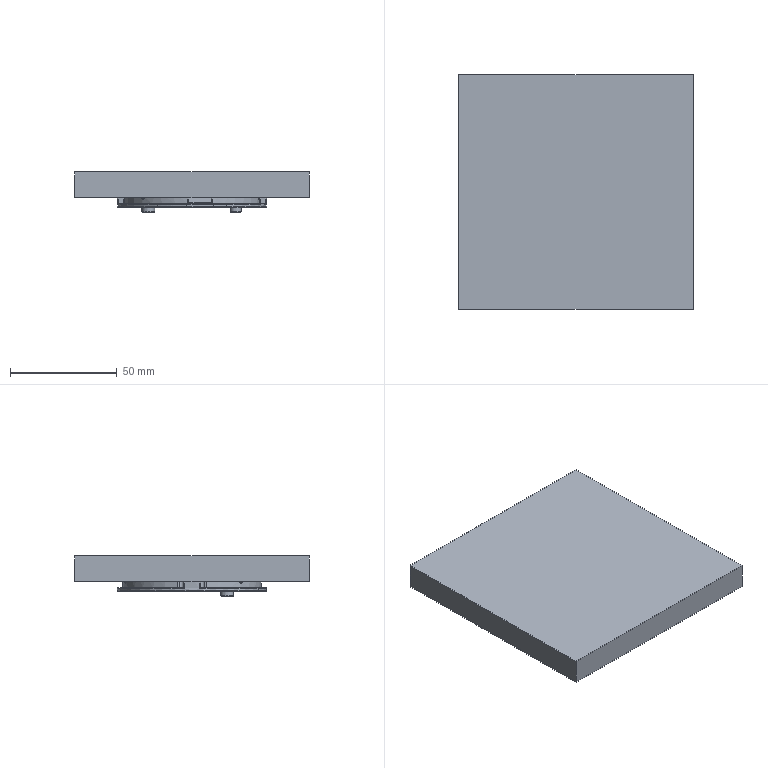NC program | NX | posted with a generic post | part box 110 x 110 x 18.8 mm
Lines 2503 to 3319 of 8004:
(ZLEVEL_PROFILE_1_COPY_1_COPY_COPY , TOOL : D2)
N4962 T02 M6
N4964 G54
N4966 G17 G0 G90 X-14.75 Y-12.131 S9500 M3
N4968 G43 Z30. H2
N4970 Z-2.8
N4972 G94 G1 Y-16.5 Z-3.029 F1000.
N4974 X-12.005 Z-3.173
N4976 X-12. Y-16.474 Z-3.174
N4978 Y-7.958 Z-3.621
N4980 X-12.053 Y-7.968 Z-3.623
N4982 X-12.32 Y-8.06 Z-3.638
N4984 X-12.965 Y-8.408 Z-3.677
N4986 X-13.537 Y-8.866 Z-3.715
N4988 X-14.015 Y-9.422 Z-3.753
N4990 X-14.384 Y-10.054 Z-3.792
N4992 X-14.632 Y-10.744 Z-3.83
N4994 X-14.75 Y-11.467 Z-3.869
N4996 Y-16.5 Z-4.132
N4998 X-12.005 Z-4.276
N5000 X-12. Y-16.474 Z-4.278
N5002 Y-12.229 Z-4.5
N5004 Y-7.958
N5006 X-12.053 Y-7.968
N5008 G3 X-14.75 Y-11.75 R4.
N5010 G1 Y-16.5
N5012 X-12.005
N5014 X-12. Y-16.474
N5016 Y-12.229
N5018 Y-8.081 Z-4.572
N5020 X-12.005 Y-7.962 Z-4.575
N5022 X-12.071 Y-7.981 Z-4.576
N5024 X-12.165 Y-8.011 Z-4.578
N5026 X-12.255 Y-8.051 Z-4.579
N5028 X-12.345 Y-8.092 Z-4.581
N5030 X-12.435 Y-8.132 Z-4.583
N5032 X-12.525 Y-8.172 Z-4.584
N5034 X-12.615 Y-8.213 Z-4.586
N5036 X-12.699 Y-8.265 Z-4.588
N5038 X-12.784 Y-8.316 Z-4.59
N5040 X-12.868 Y-8.367 Z-4.591
N5042 X-12.953 Y-8.418 Z-4.593
N5044 X-13.036 Y-8.471 Z-4.595
N5046 X-13.113 Y-8.532 Z-4.597
N5048 X-13.191 Y-8.593 Z-4.598
N5050 X-13.269 Y-8.653 Z-4.6
N5052 X-13.346 Y-8.714 Z-4.602
N5054 X-13.422 Y-8.778 Z-4.603
N5056 X-13.492 Y-8.848 Z-4.605
N5058 X-13.562 Y-8.917 Z-4.607
N5060 X-13.631 Y-8.987 Z-4.609
N5062 X-13.701 Y-9.057 Z-4.61
N5064 X-13.767 Y-9.13 Z-4.612
N5066 X-13.828 Y-9.207 Z-4.614
N5068 X-13.889 Y-9.285 Z-4.616
N5070 X-13.95 Y-9.363 Z-4.617
N5072 X-14.011 Y-9.44 Z-4.619
N5074 X-14.067 Y-9.521 Z-4.621
N5076 X-14.117 Y-9.606 Z-4.622
N5078 X-14.169 Y-9.69 Z-4.624
N5080 X-14.219 Y-9.775 Z-4.626
N5082 X-14.27 Y-9.859 Z-4.628
N5084 X-14.315 Y-9.947 Z-4.629
N5086 X-14.356 Y-10.037 Z-4.631
N5088 X-14.396 Y-10.127 Z-4.633
N5090 X-14.437 Y-10.217 Z-4.634
N5092 X-14.477 Y-10.307 Z-4.636
N5094 X-14.509 Y-10.4 Z-4.638
N5096 X-14.539 Y-10.494 Z-4.64
N5098 X-14.568 Y-10.588 Z-4.641
N5100 X-14.598 Y-10.683 Z-4.643
N5102 X-14.627 Y-10.777 Z-4.645
N5104 X-14.647 Y-10.873 Z-4.647
N5106 X-14.664 Y-10.971 Z-4.648
N5108 X-14.682 Y-11.068 Z-4.65
N5110 X-14.7 Y-11.164 Z-4.652
N5112 X-14.718 Y-11.262 Z-4.653
N5114 X-14.725 Y-11.36 Z-4.655
N5116 X-14.731 Y-11.459 Z-4.657
N5118 X-14.737 Y-11.557 Z-4.659
N5120 X-14.743 Y-11.656 Z-4.66
N5122 X-14.748 Y-11.754 Z-4.662
N5124 X-14.75 Y-11.853 Z-4.664
N5126 Y-13.927 Z-4.7
N5128 Y-16.483
N5130 X-14.745 Y-16.5
N5132 X-12.005
N5134 X-12. Y-16.474
N5136 Y-12.229
N5138 Y-8.081 Z-4.772
N5140 X-12.005 Y-7.962 Z-4.775
N5142 X-12.071 Y-7.981 Z-4.776
N5144 X-12.165 Y-8.011 Z-4.778
N5146 X-12.255 Y-8.051 Z-4.779
N5148 X-12.345 Y-8.092 Z-4.781
N5150 X-12.435 Y-8.132 Z-4.783
N5152 X-12.525 Y-8.172 Z-4.784
N5154 X-12.615 Y-8.213 Z-4.786
N5156 X-12.699 Y-8.265 Z-4.788
N5158 X-12.784 Y-8.316 Z-4.79
N5160 X-12.868 Y-8.367 Z-4.791
N5162 X-12.953 Y-8.418 Z-4.793
N5164 X-13.036 Y-8.471 Z-4.795
N5166 X-13.113 Y-8.532 Z-4.797
N5168 X-13.191 Y-8.593 Z-4.798
N5170 X-13.269 Y-8.653 Z-4.8
N5172 X-13.346 Y-8.714 Z-4.802
N5174 X-13.422 Y-8.778 Z-4.803
N5176 X-13.492 Y-8.848 Z-4.805
N5178 X-13.562 Y-8.917 Z-4.807
N5180 X-13.631 Y-8.987 Z-4.809
N5182 X-13.701 Y-9.057 Z-4.81
N5184 X-13.767 Y-9.13 Z-4.812
N5186 X-13.828 Y-9.207 Z-4.814
N5188 X-13.889 Y-9.285 Z-4.816
N5190 X-13.95 Y-9.363 Z-4.817
N5192 X-14.011 Y-9.44 Z-4.819
N5194 X-14.067 Y-9.521 Z-4.821
N5196 X-14.117 Y-9.606 Z-4.822
N5198 X-14.169 Y-9.69 Z-4.824
N5200 X-14.219 Y-9.775 Z-4.826
N5202 X-14.27 Y-9.859 Z-4.828
N5204 X-14.315 Y-9.947 Z-4.829
N5206 X-14.356 Y-10.037 Z-4.831
N5208 X-14.396 Y-10.127 Z-4.833
N5210 X-14.437 Y-10.217 Z-4.834
N5212 X-14.477 Y-10.307 Z-4.836
N5214 X-14.509 Y-10.4 Z-4.838
N5216 X-14.539 Y-10.494 Z-4.84
N5218 X-14.568 Y-10.588 Z-4.841
N5220 X-14.598 Y-10.683 Z-4.843
N5222 X-14.627 Y-10.777 Z-4.845
N5224 X-14.647 Y-10.873 Z-4.847
N5226 X-14.664 Y-10.971 Z-4.848
N5228 X-14.682 Y-11.068 Z-4.85
N5230 X-14.7 Y-11.164 Z-4.852
N5232 X-14.718 Y-11.262 Z-4.853
N5234 X-14.725 Y-11.36 Z-4.855
N5236 X-14.731 Y-11.459 Z-4.857
N5238 X-14.737 Y-11.557 Z-4.859
N5240 X-14.743 Y-11.656 Z-4.86
N5242 X-14.748 Y-11.754 Z-4.862
N5244 X-14.75 Y-11.853 Z-4.864
N5246 Y-13.927 Z-4.9
N5248 Y-16.483
N5250 X-14.745 Y-16.5
N5252 X-12.005
N5254 X-12. Y-16.474
N5256 Y-12.229
N5258 Y-8.081 Z-4.972
N5260 X-12.005 Y-7.962 Z-4.975
N5262 X-12.071 Y-7.981 Z-4.976
N5264 X-12.165 Y-8.011 Z-4.978
N5266 X-12.255 Y-8.051 Z-4.979
N5268 X-12.345 Y-8.092 Z-4.981
N5270 X-12.435 Y-8.132 Z-4.983
N5272 X-12.525 Y-8.172 Z-4.984
N5274 X-12.615 Y-8.213 Z-4.986
N5276 X-12.699 Y-8.265 Z-4.988
N5278 X-12.784 Y-8.316 Z-4.99
N5280 X-12.868 Y-8.367 Z-4.991
N5282 X-12.953 Y-8.418 Z-4.993
N5284 X-13.036 Y-8.471 Z-4.995
N5286 X-13.113 Y-8.532 Z-4.997
N5288 X-13.191 Y-8.593 Z-4.998
N5290 X-13.269 Y-8.653 Z-5.
N5292 X-13.346 Y-8.714 Z-5.002
N5294 X-13.422 Y-8.778 Z-5.003
N5296 X-13.492 Y-8.848 Z-5.005
N5298 X-13.562 Y-8.917 Z-5.007
N5300 X-13.631 Y-8.987 Z-5.009
N5302 X-13.701 Y-9.057 Z-5.01
N5304 X-13.767 Y-9.13 Z-5.012
N5306 X-13.828 Y-9.207 Z-5.014
N5308 X-13.889 Y-9.285 Z-5.016
N5310 X-13.95 Y-9.363 Z-5.017
N5312 X-14.011 Y-9.44 Z-5.019
N5314 X-14.067 Y-9.521 Z-5.021
N5316 X-14.117 Y-9.606 Z-5.022
N5318 X-14.169 Y-9.69 Z-5.024
N5320 X-14.219 Y-9.775 Z-5.026
N5322 X-14.27 Y-9.859 Z-5.028
N5324 X-14.315 Y-9.947 Z-5.029
N5326 X-14.356 Y-10.037 Z-5.031
N5328 X-14.396 Y-10.127 Z-5.033
N5330 X-14.437 Y-10.217 Z-5.034
N5332 X-14.477 Y-10.307 Z-5.036
N5334 X-14.509 Y-10.4 Z-5.038
N5336 X-14.539 Y-10.494 Z-5.04
N5338 X-14.568 Y-10.588 Z-5.041
N5340 X-14.598 Y-10.683 Z-5.043
N5342 X-14.627 Y-10.777 Z-5.045
N5344 X-14.647 Y-10.873 Z-5.047
N5346 X-14.664 Y-10.971 Z-5.048
N5348 X-14.682 Y-11.068 Z-5.05
N5350 X-14.7 Y-11.165 Z-5.052
N5352 X-14.718 Y-11.262 Z-5.053
N5354 X-14.724 Y-11.36 Z-5.055
N5356 X-14.731 Y-11.459 Z-5.057
N5358 X-14.737 Y-11.557 Z-5.059
N5360 X-14.743 Y-11.656 Z-5.06
N5362 X-14.748 Y-11.754 Z-5.062
N5364 X-14.75 Y-11.853 Z-5.064
N5366 Y-13.927 Z-5.1
N5368 Y-16.483
N5370 X-14.745 Y-16.5
N5372 X-12.005
N5374 X-12. Y-16.474
N5376 Y-12.229
N5378 Y-8.081 Z-5.172
N5380 X-12.005 Y-7.962 Z-5.175
N5382 X-12.071 Y-7.981 Z-5.176
N5384 X-12.165 Y-8.011 Z-5.178
N5386 X-12.255 Y-8.051 Z-5.179
N5388 X-12.345 Y-8.092 Z-5.181
N5390 X-12.435 Y-8.132 Z-5.183
N5392 X-12.525 Y-8.172 Z-5.184
N5394 X-12.615 Y-8.213 Z-5.186
N5396 X-12.699 Y-8.265 Z-5.188
N5398 X-12.784 Y-8.316 Z-5.19
N5400 X-12.868 Y-8.367 Z-5.191
N5402 X-12.953 Y-8.418 Z-5.193
N5404 X-13.036 Y-8.471 Z-5.195
N5406 X-13.113 Y-8.532 Z-5.197
N5408 X-13.191 Y-8.593 Z-5.198
N5410 X-13.269 Y-8.653 Z-5.2
N5412 X-13.346 Y-8.714 Z-5.202
N5414 X-13.422 Y-8.778 Z-5.203
N5416 X-13.491 Y-8.848 Z-5.205
N5418 X-13.562 Y-8.917 Z-5.207
N5420 X-13.631 Y-8.987 Z-5.209
N5422 X-13.701 Y-9.057 Z-5.21
N5424 X-13.767 Y-9.13 Z-5.212
N5426 X-13.828 Y-9.207 Z-5.214
N5428 X-13.889 Y-9.285 Z-5.216
N5430 X-13.95 Y-9.363 Z-5.217
N5432 X-14.011 Y-9.44 Z-5.219
N5434 X-14.067 Y-9.521 Z-5.221
N5436 X-14.117 Y-9.606 Z-5.222
N5438 X-14.169 Y-9.69 Z-5.224
N5440 X-14.219 Y-9.775 Z-5.226
N5442 X-14.27 Y-9.859 Z-5.228
N5444 X-14.315 Y-9.947 Z-5.229
N5446 X-14.356 Y-10.037 Z-5.231
N5448 X-14.396 Y-10.127 Z-5.233
N5450 X-14.437 Y-10.217 Z-5.234
N5452 X-14.477 Y-10.307 Z-5.236
N5454 X-14.509 Y-10.4 Z-5.238
N5456 X-14.539 Y-10.494 Z-5.24
N5458 X-14.568 Y-10.588 Z-5.241
N5460 X-14.598 Y-10.683 Z-5.243
N5462 X-14.627 Y-10.777 Z-5.245
N5464 X-14.647 Y-10.873 Z-5.247
N5466 X-14.664 Y-10.971 Z-5.248
N5468 X-14.682 Y-11.068 Z-5.25
N5470 X-14.7 Y-11.165 Z-5.252
N5472 X-14.718 Y-11.262 Z-5.253
N5474 X-14.724 Y-11.36 Z-5.255
N5476 X-14.731 Y-11.459 Z-5.257
N5478 X-14.737 Y-11.557 Z-5.259
N5480 X-14.743 Y-11.656 Z-5.26
N5482 X-14.748 Y-11.754 Z-5.262
N5484 X-14.75 Y-11.853 Z-5.264
N5486 Y-13.927 Z-5.3
N5488 Y-16.483
N5490 X-14.745 Y-16.5
N5492 X-12.005
N5494 X-12. Y-16.474
N5496 Y-12.229
N5498 Y-8.081 Z-5.372
N5500 X-12.005 Y-7.962 Z-5.375
N5502 X-12.071 Y-7.981 Z-5.376
N5504 X-12.165 Y-8.011 Z-5.378
N5506 X-12.255 Y-8.051 Z-5.379
N5508 X-12.346 Y-8.091 Z-5.381
N5510 X-12.435 Y-8.132 Z-5.383
N5512 X-12.525 Y-8.172 Z-5.384
N5514 X-12.615 Y-8.213 Z-5.386
N5516 X-12.699 Y-8.265 Z-5.388
N5518 X-12.784 Y-8.316 Z-5.39
N5520 X-12.868 Y-8.367 Z-5.391
N5522 X-12.953 Y-8.418 Z-5.393
N5524 X-13.036 Y-8.471 Z-5.395
N5526 X-13.113 Y-8.532 Z-5.397
N5528 X-13.191 Y-8.593 Z-5.398
N5530 X-13.269 Y-8.653 Z-5.4
N5532 X-13.346 Y-8.714 Z-5.402
N5534 X-13.422 Y-8.778 Z-5.403
N5536 X-13.491 Y-8.848 Z-5.405
N5538 X-13.562 Y-8.917 Z-5.407
N5540 X-13.631 Y-8.987 Z-5.409
N5542 X-13.701 Y-9.057 Z-5.41
N5544 X-13.767 Y-9.13 Z-5.412
N5546 X-13.828 Y-9.207 Z-5.414
N5548 X-13.889 Y-9.285 Z-5.416
N5550 X-13.95 Y-9.363 Z-5.417
N5552 X-14.011 Y-9.44 Z-5.419
N5554 X-14.067 Y-9.521 Z-5.421
N5556 X-14.117 Y-9.606 Z-5.422
N5558 X-14.169 Y-9.69 Z-5.424
N5560 X-14.219 Y-9.775 Z-5.426
N5562 X-14.27 Y-9.859 Z-5.428
N5564 X-14.315 Y-9.947 Z-5.429
N5566 X-14.356 Y-10.037 Z-5.431
N5568 X-14.396 Y-10.127 Z-5.433
N5570 X-14.437 Y-10.217 Z-5.434
N5572 X-14.477 Y-10.307 Z-5.436
N5574 X-14.509 Y-10.4 Z-5.438
N5576 X-14.539 Y-10.495 Z-5.44
N5578 X-14.568 Y-10.588 Z-5.441
N5580 X-14.597 Y-10.683 Z-5.443
N5582 X-14.627 Y-10.777 Z-5.445
N5584 X-14.647 Y-10.873 Z-5.447
N5586 X-14.664 Y-10.971 Z-5.448
N5588 X-14.682 Y-11.068 Z-5.45
N5590 X-14.7 Y-11.165 Z-5.452
N5592 X-14.718 Y-11.262 Z-5.453
N5594 X-14.724 Y-11.36 Z-5.455
N5596 X-14.731 Y-11.459 Z-5.457
N5598 X-14.737 Y-11.557 Z-5.459
N5600 X-14.743 Y-11.656 Z-5.46
N5602 X-14.748 Y-11.754 Z-5.462
N5604 X-14.75 Y-11.853 Z-5.464
N5606 Y-13.927 Z-5.5
N5608 Y-16.483
N5610 X-14.745 Y-16.5
N5612 X-12.005
N5614 X-12. Y-16.474
N5616 Y-12.229
N5618 Y-8.081 Z-5.572
N5620 X-12.005 Y-7.962 Z-5.575
N5622 X-12.071 Y-7.981 Z-5.576
N5624 X-12.165 Y-8.011 Z-5.578
N5626 X-12.255 Y-8.051 Z-5.579
N5628 X-12.346 Y-8.091 Z-5.581
N5630 X-12.435 Y-8.132 Z-5.583
N5632 X-12.525 Y-8.172 Z-5.584
N5634 X-12.615 Y-8.213 Z-5.586
N5636 X-12.699 Y-8.265 Z-5.588
N5638 X-12.784 Y-8.316 Z-5.59
N5640 X-12.868 Y-8.367 Z-5.591
N5642 X-12.953 Y-8.418 Z-5.593
N5644 X-13.036 Y-8.471 Z-5.595
N5646 X-13.113 Y-8.532 Z-5.597
N5648 X-13.191 Y-8.593 Z-5.598
N5650 X-13.269 Y-8.653 Z-5.6
N5652 X-13.346 Y-8.714 Z-5.602
N5654 X-13.422 Y-8.778 Z-5.603
N5656 X-13.491 Y-8.848 Z-5.605
N5658 X-13.562 Y-8.917 Z-5.607
N5660 X-13.631 Y-8.987 Z-5.609
N5662 X-13.701 Y-9.057 Z-5.61
N5664 X-13.767 Y-9.13 Z-5.612
N5666 X-13.828 Y-9.207 Z-5.614
N5668 X-13.889 Y-9.285 Z-5.616
N5670 X-13.95 Y-9.363 Z-5.617
N5672 X-14.011 Y-9.44 Z-5.619
N5674 X-14.067 Y-9.522 Z-5.621
N5676 X-14.117 Y-9.606 Z-5.622
N5678 X-14.169 Y-9.69 Z-5.624
N5680 X-14.219 Y-9.775 Z-5.626
N5682 X-14.27 Y-9.859 Z-5.628
N5684 X-14.315 Y-9.947 Z-5.629
N5686 X-14.356 Y-10.037 Z-5.631
N5688 X-14.396 Y-10.127 Z-5.633
N5690 X-14.437 Y-10.217 Z-5.634
N5692 X-14.477 Y-10.307 Z-5.636
N5694 X-14.509 Y-10.4 Z-5.638
N5696 X-14.539 Y-10.495 Z-5.64
N5698 X-14.568 Y-10.589 Z-5.641
N5700 X-14.597 Y-10.683 Z-5.643
N5702 X-14.627 Y-10.777 Z-5.645
N5704 X-14.647 Y-10.874 Z-5.647
N5706 X-14.664 Y-10.971 Z-5.648
N5708 X-14.682 Y-11.068 Z-5.65
N5710 X-14.7 Y-11.165 Z-5.652
N5712 X-14.718 Y-11.262 Z-5.653
N5714 X-14.724 Y-11.36 Z-5.655
N5716 X-14.731 Y-11.459 Z-5.657
N5718 X-14.737 Y-11.557 Z-5.659
N5720 X-14.743 Y-11.656 Z-5.66
N5722 X-14.748 Y-11.754 Z-5.662
N5724 X-14.75 Y-11.853 Z-5.664
N5726 Y-13.927 Z-5.7
N5728 Y-16.483
N5730 X-14.745 Y-16.5
N5732 X-12.005
N5734 X-12. Y-16.474
N5736 Y-12.229
N5738 Y-8.081 Z-5.772
N5740 X-12.005 Y-7.962 Z-5.775
N5742 X-12.071 Y-7.981 Z-5.776
N5744 X-12.165 Y-8.011 Z-5.778
N5746 X-12.255 Y-8.051 Z-5.779
N5748 X-12.346 Y-8.091 Z-5.781
N5750 X-12.435 Y-8.132 Z-5.783
N5752 X-12.525 Y-8.172 Z-5.784
N5754 X-12.615 Y-8.213 Z-5.786
N5756 X-12.699 Y-8.265 Z-5.788
N5758 X-12.784 Y-8.316 Z-5.79
N5760 X-12.868 Y-8.367 Z-5.791
N5762 X-12.953 Y-8.418 Z-5.793
N5764 X-13.036 Y-8.471 Z-5.795
N5766 X-13.113 Y-8.532 Z-5.797
N5768 X-13.191 Y-8.593 Z-5.798
N5770 X-13.269 Y-8.653 Z-5.8
N5772 X-13.346 Y-8.714 Z-5.802
N5774 X-13.422 Y-8.778 Z-5.803
N5776 X-13.491 Y-8.848 Z-5.805
N5778 X-13.562 Y-8.917 Z-5.807
N5780 X-13.631 Y-8.987 Z-5.809
N5782 X-13.701 Y-9.057 Z-5.81
N5784 X-13.767 Y-9.13 Z-5.812
N5786 X-13.828 Y-9.207 Z-5.814
N5788 X-13.889 Y-9.285 Z-5.816
N5790 X-13.95 Y-9.363 Z-5.817
N5792 X-14.011 Y-9.44 Z-5.819
N5794 X-14.067 Y-9.522 Z-5.821
N5796 X-14.117 Y-9.606 Z-5.822
N5798 X-14.169 Y-9.69 Z-5.824
N5800 X-14.219 Y-9.775 Z-5.826
N5802 X-14.27 Y-9.859 Z-5.828
N5804 X-14.315 Y-9.947 Z-5.829
N5806 X-14.356 Y-10.037 Z-5.831
N5808 X-14.396 Y-10.127 Z-5.833
N5810 X-14.437 Y-10.217 Z-5.834
N5812 X-14.477 Y-10.307 Z-5.836
N5814 X-14.509 Y-10.4 Z-5.838
N5816 X-14.539 Y-10.494 Z-5.84
N5818 X-14.568 Y-10.589 Z-5.841
N5820 X-14.597 Y-10.683 Z-5.843
N5822 X-14.627 Y-10.777 Z-5.845
N5824 X-14.647 Y-10.874 Z-5.847
N5826 X-14.664 Y-10.971 Z-5.848
N5828 X-14.682 Y-11.068 Z-5.85
N5830 X-14.7 Y-11.165 Z-5.852
N5832 X-14.718 Y-11.262 Z-5.853
N5834 X-14.724 Y-11.36 Z-5.855
N5836 X-14.731 Y-11.459 Z-5.857
N5838 X-14.736 Y-11.557 Z-5.859
N5840 X-14.743 Y-11.656 Z-5.86
N5842 X-14.748 Y-11.754 Z-5.862
N5844 X-14.75 Y-11.853 Z-5.864
N5846 Y-13.927 Z-5.9
N5848 Y-16.483
N5850 X-14.745 Y-16.5
N5852 X-12.005
N5854 X-12. Y-16.474
N5856 Y-12.229
N5858 Y-8.081 Z-5.972
N5860 X-12.005 Y-7.962 Z-5.975
N5862 X-12.071 Y-7.981 Z-5.976
N5864 X-12.165 Y-8.011 Z-5.978
N5866 X-12.255 Y-8.051 Z-5.979
N5868 X-12.346 Y-8.091 Z-5.981
N5870 X-12.435 Y-8.132 Z-5.983
N5872 X-12.525 Y-8.172 Z-5.984
N5874 X-12.615 Y-8.213 Z-5.986
N5876 X-12.699 Y-8.265 Z-5.988
N5878 X-12.784 Y-8.316 Z-5.99
N5880 X-12.868 Y-8.367 Z-5.991
N5882 X-12.953 Y-8.418 Z-5.993
N5884 X-13.036 Y-8.471 Z-5.995
N5886 X-13.113 Y-8.532 Z-5.997
N5888 X-13.191 Y-8.593 Z-5.998
N5890 X-13.269 Y-8.653 Z-6.
N5892 X-13.346 Y-8.714 Z-6.002
N5894 X-13.422 Y-8.778 Z-6.003
N5896 X-13.491 Y-8.848 Z-6.005
N5898 X-13.562 Y-8.917 Z-6.007
N5900 X-13.631 Y-8.987 Z-6.009
N5902 X-13.701 Y-9.057 Z-6.01
N5904 X-13.767 Y-9.13 Z-6.012
N5906 X-13.828 Y-9.207 Z-6.014
N5908 X-13.889 Y-9.285 Z-6.016
N5910 X-13.95 Y-9.363 Z-6.017
N5912 X-14.011 Y-9.44 Z-6.019
N5914 X-14.067 Y-9.522 Z-6.021
N5916 X-14.117 Y-9.606 Z-6.022
N5918 X-14.169 Y-9.69 Z-6.024
N5920 X-14.219 Y-9.775 Z-6.026
N5922 X-14.27 Y-9.859 Z-6.028
N5924 X-14.315 Y-9.947 Z-6.029
N5926 X-14.356 Y-10.037 Z-6.031
N5928 X-14.396 Y-10.127 Z-6.033
N5930 X-14.437 Y-10.217 Z-6.034
N5932 X-14.477 Y-10.307 Z-6.036
N5934 X-14.509 Y-10.4 Z-6.038
N5936 X-14.539 Y-10.494 Z-6.04
N5938 X-14.568 Y-10.589 Z-6.041
N5940 X-14.597 Y-10.683 Z-6.043
N5942 X-14.627 Y-10.777 Z-6.045
N5944 X-14.647 Y-10.874 Z-6.047
N5946 X-14.664 Y-10.971 Z-6.048
N5948 X-14.682 Y-11.068 Z-6.05
N5950 X-14.7 Y-11.165 Z-6.052
N5952 X-14.718 Y-11.262 Z-6.053
N5954 X-14.724 Y-11.36 Z-6.055
N5956 X-14.731 Y-11.459 Z-6.057
N5958 X-14.736 Y-11.557 Z-6.059
N5960 X-14.743 Y-11.656 Z-6.06
N5962 X-14.748 Y-11.754 Z-6.062
N5964 X-14.75 Y-11.853 Z-6.064
N5966 Y-13.927 Z-6.1
N5968 Y-16.483
N5970 X-14.745 Y-16.5
N5972 X-12.005
N5974 X-12. Y-16.474
N5976 Y-12.229
N5978 Y-8.081 Z-6.172
N5980 X-12.005 Y-7.962 Z-6.175
N5982 X-12.071 Y-7.981 Z-6.176
N5984 X-12.165 Y-8.011 Z-6.178
N5986 X-12.255 Y-8.051 Z-6.179
N5988 X-12.346 Y-8.091 Z-6.181
N5990 X-12.435 Y-8.132 Z-6.183
N5992 X-12.525 Y-8.172 Z-6.184
N5994 X-12.615 Y-8.214 Z-6.186
N5996 X-12.699 Y-8.265 Z-6.188
N5998 X-12.784 Y-8.316 Z-6.19
N6000 X-12.868 Y-8.367 Z-6.191
N6002 X-12.953 Y-8.418 Z-6.193
N6004 X-13.036 Y-8.471 Z-6.195
N6006 X-13.113 Y-8.532 Z-6.197
N6008 X-13.191 Y-8.593 Z-6.198
N6010 X-13.269 Y-8.653 Z-6.2
N6012 X-13.346 Y-8.714 Z-6.202
N6014 X-13.422 Y-8.778 Z-6.203
N6016 X-13.491 Y-8.848 Z-6.205
N6018 X-13.562 Y-8.917 Z-6.207
N6020 X-13.631 Y-8.987 Z-6.209
N6022 X-13.701 Y-9.057 Z-6.21
N6024 X-13.767 Y-9.13 Z-6.212
N6026 X-13.828 Y-9.207 Z-6.214
N6028 X-13.889 Y-9.285 Z-6.216
N6030 X-13.95 Y-9.363 Z-6.217
N6032 X-14.011 Y-9.44 Z-6.219
N6034 X-14.067 Y-9.522 Z-6.221
N6036 X-14.117 Y-9.606 Z-6.222
N6038 X-14.169 Y-9.69 Z-6.224
N6040 X-14.219 Y-9.775 Z-6.226
N6042 X-14.27 Y-9.86 Z-6.228
N6044 X-14.315 Y-9.947 Z-6.229
N6046 X-14.356 Y-10.037 Z-6.231
N6048 X-14.396 Y-10.127 Z-6.233
N6050 X-14.437 Y-10.217 Z-6.234
N6052 X-14.477 Y-10.307 Z-6.236
N6054 X-14.509 Y-10.4 Z-6.238
N6056 X-14.539 Y-10.494 Z-6.24
N6058 X-14.568 Y-10.589 Z-6.241
N6060 X-14.597 Y-10.683 Z-6.243
N6062 X-14.627 Y-10.777 Z-6.245
N6064 X-14.647 Y-10.874 Z-6.247
N6066 X-14.664 Y-10.971 Z-6.248
N6068 X-14.682 Y-11.068 Z-6.25
N6070 X-14.7 Y-11.165 Z-6.252
N6072 X-14.718 Y-11.262 Z-6.253
N6074 X-14.724 Y-11.36 Z-6.255
N6076 X-14.731 Y-11.459 Z-6.257
N6078 X-14.736 Y-11.557 Z-6.259
N6080 X-14.743 Y-11.656 Z-6.26
N6082 X-14.748 Y-11.754 Z-6.262
N6084 X-14.75 Y-11.853 Z-6.264
N6086 Y-13.927 Z-6.3
N6088 Y-16.483
N6090 X-14.745 Y-16.5
N6092 X-12.005
N6094 X-12. Y-16.474
N6096 Y-12.229
N6098 Y-8.081 Z-6.372
N6100 X-12.005 Y-7.962 Z-6.375
N6102 X-12.071 Y-7.981 Z-6.376
N6104 X-12.165 Y-8.011 Z-6.378
N6106 X-12.256 Y-8.051 Z-6.379
N6108 X-12.346 Y-8.091 Z-6.381
N6110 X-12.435 Y-8.132 Z-6.383
N6112 X-12.525 Y-8.172 Z-6.384
N6114 X-12.615 Y-8.214 Z-6.386
N6116 X-12.699 Y-8.265 Z-6.388
N6118 X-12.784 Y-8.316 Z-6.39
N6120 X-12.868 Y-8.367 Z-6.391
N6122 X-12.953 Y-8.418 Z-6.393
N6124 X-13.036 Y-8.471 Z-6.395
N6126 X-13.114 Y-8.532 Z-6.397
N6128 X-13.191 Y-8.593 Z-6.398
N6130 X-13.269 Y-8.653 Z-6.4
N6132 X-13.346 Y-8.714 Z-6.402
N6134 X-13.422 Y-8.778 Z-6.403
N6136 X-13.491 Y-8.848 Z-6.405
N6138 X-13.562 Y-8.917 Z-6.407
N6140 X-13.631 Y-8.987 Z-6.409
N6142 X-13.701 Y-9.057 Z-6.41
N6144 X-13.767 Y-9.13 Z-6.412
N6146 X-13.828 Y-9.207 Z-6.414
N6148 X-13.889 Y-9.285 Z-6.416
N6150 X-13.95 Y-9.363 Z-6.417
N6152 X-14.011 Y-9.44 Z-6.419
N6154 X-14.067 Y-9.522 Z-6.421
N6156 X-14.117 Y-9.606 Z-6.422
N6158 X-14.169 Y-9.69 Z-6.424
N6160 X-14.22 Y-9.775 Z-6.426
N6162 X-14.27 Y-9.86 Z-6.428
N6164 X-14.315 Y-9.947 Z-6.429
N6166 X-14.356 Y-10.037 Z-6.431
N6168 X-14.396 Y-10.127 Z-6.433
N6170 X-14.437 Y-10.217 Z-6.434
N6172 X-14.477 Y-10.307 Z-6.436
N6174 X-14.509 Y-10.4 Z-6.438
N6176 X-14.539 Y-10.494 Z-6.44
N6178 X-14.568 Y-10.589 Z-6.441
N6180 X-14.597 Y-10.683 Z-6.443
N6182 X-14.627 Y-10.777 Z-6.445
N6184 X-14.647 Y-10.874 Z-6.447
N6186 X-14.664 Y-10.971 Z-6.448
N6188 X-14.682 Y-11.068 Z-6.45
N6190 X-14.7 Y-11.165 Z-6.452
N6192 X-14.718 Y-11.262 Z-6.453
N6194 X-14.724 Y-11.36 Z-6.455
N6196 X-14.731 Y-11.459 Z-6.457
N6198 X-14.736 Y-11.557 Z-6.459
N6200 X-14.743 Y-11.656 Z-6.46
N6202 X-14.748 Y-11.754 Z-6.462
N6204 X-14.75 Y-11.853 Z-6.464
N6206 Y-13.927 Z-6.5
N6208 Y-16.483
N6210 X-14.745 Y-16.5
N6212 X-12.005
N6214 X-12. Y-16.474
N6216 Y-12.229
N6218 Y-8.081 Z-6.572
N6220 X-12.005 Y-7.962 Z-6.575
N6222 X-12.071 Y-7.981 Z-6.576
N6224 X-12.165 Y-8.011 Z-6.578
N6226 X-12.256 Y-8.051 Z-6.579
N6228 X-12.346 Y-8.091 Z-6.581
N6230 X-12.435 Y-8.132 Z-6.583
N6232 X-12.525 Y-8.172 Z-6.584
N6234 X-12.615 Y-8.214 Z-6.586
N6236 X-12.699 Y-8.265 Z-6.588
N6238 X-12.784 Y-8.316 Z-6.59
N6240 X-12.868 Y-8.367 Z-6.591
N6242 X-12.953 Y-8.418 Z-6.593
N6244 X-13.036 Y-8.471 Z-6.595
N6246 X-13.114 Y-8.532 Z-6.597
N6248 X-13.191 Y-8.593 Z-6.598
N6250 X-13.269 Y-8.653 Z-6.6
N6252 X-13.346 Y-8.715 Z-6.602
N6254 X-13.422 Y-8.778 Z-6.603
N6256 X-13.491 Y-8.848 Z-6.605
N6258 X-13.562 Y-8.917 Z-6.607
N6260 X-13.631 Y-8.987 Z-6.609
N6262 X-13.701 Y-9.057 Z-6.61
N6264 X-13.767 Y-9.13 Z-6.612
N6266 X-13.828 Y-9.207 Z-6.614
N6268 X-13.889 Y-9.285 Z-6.616
N6270 X-13.95 Y-9.363 Z-6.617
N6272 X-14.011 Y-9.44 Z-6.619
N6274 X-14.067 Y-9.522 Z-6.621
N6276 X-14.117 Y-9.606 Z-6.622
N6278 X-14.169 Y-9.69 Z-6.624
N6280 X-14.22 Y-9.775 Z-6.626
N6282 X-14.27 Y-9.86 Z-6.628
N6284 X-14.315 Y-9.947 Z-6.629
N6286 X-14.356 Y-10.037 Z-6.631
N6288 X-14.396 Y-10.127 Z-6.633
N6290 X-14.437 Y-10.217 Z-6.634
N6292 X-14.477 Y-10.307 Z-6.636
N6294 X-14.509 Y-10.4 Z-6.638
N6296 X-14.539 Y-10.494 Z-6.64
N6298 X-14.568 Y-10.589 Z-6.641
N6300 X-14.597 Y-10.683 Z-6.643
N6302 X-14.627 Y-10.777 Z-6.645
N6304 X-14.647 Y-10.874 Z-6.647
N6306 X-14.664 Y-10.971 Z-6.648
N6308 X-14.682 Y-11.068 Z-6.65
N6310 X-14.7 Y-11.165 Z-6.652
N6312 X-14.718 Y-11.262 Z-6.653
N6314 X-14.724 Y-11.36 Z-6.655
N6316 X-14.731 Y-11.459 Z-6.657
N6318 X-14.736 Y-11.557 Z-6.659
N6320 X-14.743 Y-11.656 Z-6.66
N6322 X-14.748 Y-11.754 Z-6.662
N6324 X-14.75 Y-11.853 Z-6.664
N6326 Y-13.927 Z-6.7
N6328 Y-16.483
N6330 X-14.745 Y-16.5
N6332 X-12.005
N6334 X-12. Y-16.474
N6336 Y-12.229
N6338 Y-8.081 Z-6.772
N6340 X-12.005 Y-7.962 Z-6.775
N6342 X-12.071 Y-7.981 Z-6.776
N6344 X-12.165 Y-8.011 Z-6.778
N6346 X-12.256 Y-8.051 Z-6.779
N6348 X-12.346 Y-8.091 Z-6.781
N6350 X-12.435 Y-8.132 Z-6.783
N6352 X-12.525 Y-8.172 Z-6.784
N6354 X-12.615 Y-8.214 Z-6.786
N6356 X-12.699 Y-8.265 Z-6.788
N6358 X-12.784 Y-8.316 Z-6.79
N6360 X-12.868 Y-8.367 Z-6.791
N6362 X-12.953 Y-8.418 Z-6.793
N6364 X-13.036 Y-8.471 Z-6.795
N6366 X-13.114 Y-8.532 Z-6.797
N6368 X-13.191 Y-8.593 Z-6.798
N6370 X-13.269 Y-8.653 Z-6.8
N6372 X-13.346 Y-8.715 Z-6.802
N6374 X-13.422 Y-8.778 Z-6.803
N6376 X-13.491 Y-8.848 Z-6.805
N6378 X-13.562 Y-8.917 Z-6.807
N6380 X-13.631 Y-8.987 Z-6.809
N6382 X-13.701 Y-9.057 Z-6.81
N6384 X-13.767 Y-9.13 Z-6.812
N6386 X-13.828 Y-9.207 Z-6.814
N6388 X-13.889 Y-9.285 Z-6.816
N6390 X-13.95 Y-9.363 Z-6.817
N6392 X-14.011 Y-9.44 Z-6.819
N6394 X-14.067 Y-9.522 Z-6.821
N6396 X-14.117 Y-9.606 Z-6.822
N6398 X-14.169 Y-9.691 Z-6.824
N6400 X-14.22 Y-9.775 Z-6.826
N6402 X-14.27 Y-9.86 Z-6.828
N6404 X-14.315 Y-9.947 Z-6.829
N6406 X-14.356 Y-10.037 Z-6.831
N6408 X-14.396 Y-10.127 Z-6.833
N6410 X-14.437 Y-10.217 Z-6.834
N6412 X-14.477 Y-10.307 Z-6.836
N6414 X-14.509 Y-10.4 Z-6.838
N6416 X-14.539 Y-10.494 Z-6.84
N6418 X-14.568 Y-10.589 Z-6.841
N6420 X-14.597 Y-10.683 Z-6.843
N6422 X-14.627 Y-10.777 Z-6.845
N6424 X-14.647 Y-10.874 Z-6.847
N6426 X-14.664 Y-10.971 Z-6.848
N6428 X-14.683 Y-11.068 Z-6.85
N6430 X-14.7 Y-11.165 Z-6.852
N6432 X-14.718 Y-11.262 Z-6.853
N6434 X-14.724 Y-11.36 Z-6.855
N6436 X-14.731 Y-11.459 Z-6.857
N6438 X-14.736 Y-11.557 Z-6.859
N6440 X-14.743 Y-11.656 Z-6.86
N6442 X-14.748 Y-11.754 Z-6.862
N6444 X-14.75 Y-11.853 Z-6.864
N6446 Y-13.927 Z-6.9
N6448 Y-16.483
N6450 X-14.745 Y-16.5
N6452 X-12.005
N6454 X-12. Y-16.474
N6456 Y-12.229
N6458 Y-8.081 Z-6.972
N6460 X-12.006 Y-7.962 Z-6.975
N6462 X-12.071 Y-7.981 Z-6.976
N6464 X-12.165 Y-8.011 Z-6.978
N6466 X-12.256 Y-8.051 Z-6.979
N6468 X-12.346 Y-8.091 Z-6.981
N6470 X-12.435 Y-8.132 Z-6.983
N6472 X-12.525 Y-8.172 Z-6.984
N6474 X-12.615 Y-8.214 Z-6.986
N6476 X-12.699 Y-8.265 Z-6.988
N6478 X-12.784 Y-8.316 Z-6.99
N6480 X-12.868 Y-8.367 Z-6.991
N6482 X-12.953 Y-8.418 Z-6.993
N6484 X-13.036 Y-8.471 Z-6.995
N6486 X-13.114 Y-8.532 Z-6.997
N6488 X-13.191 Y-8.593 Z-6.998
N6490 X-13.269 Y-8.653 Z-7.
N6492 X-13.346 Y-8.715 Z-7.002
N6494 X-13.422 Y-8.778 Z-7.003
N6496 X-13.491 Y-8.848 Z-7.005
N6498 X-13.562 Y-8.917 Z-7.007
N6500 X-13.631 Y-8.987 Z-7.009
N6502 X-13.701 Y-9.057 Z-7.01
N6504 X-13.767 Y-9.13 Z-7.012
N6506 X-13.828 Y-9.207 Z-7.014
N6508 X-13.889 Y-9.285 Z-7.016
N6510 X-13.95 Y-9.363 Z-7.017
N6512 X-14.011 Y-9.441 Z-7.019
N6514 X-14.067 Y-9.522 Z-7.021
N6516 X-14.117 Y-9.606 Z-7.022
N6518 X-14.169 Y-9.691 Z-7.024
N6520 X-14.22 Y-9.775 Z-7.026
N6522 X-14.27 Y-9.86 Z-7.028
N6524 X-14.315 Y-9.947 Z-7.029
N6526 X-14.356 Y-10.037 Z-7.031
N6528 X-14.396 Y-10.127 Z-7.033
N6530 X-14.437 Y-10.217 Z-7.034
N6532 X-14.477 Y-10.307 Z-7.036
N6534 X-14.509 Y-10.401 Z-7.038
N6536 X-14.539 Y-10.494 Z-7.04
N6538 X-14.568 Y-10.589 Z-7.041
N6540 X-14.597 Y-10.683 Z-7.043
N6542 X-14.627 Y-10.777 Z-7.045
N6544 X-14.647 Y-10.874 Z-7.047
N6546 X-14.664 Y-10.971 Z-7.048
N6548 X-14.683 Y-11.068 Z-7.05
N6550 X-14.7 Y-11.165 Z-7.052
N6552 X-14.718 Y-11.262 Z-7.053
N6554 X-14.724 Y-11.36 Z-7.055
N6556 X-14.731 Y-11.459 Z-7.057
N6558 X-14.736 Y-11.557 Z-7.059
N6560 X-14.743 Y-11.656 Z-7.06
N6562 X-14.748 Y-11.754 Z-7.062
N6564 X-14.75 Y-11.853 Z-7.064
N6566 Y-13.927 Z-7.1
N6568 Y-16.483
N6570 X-14.745 Y-16.5
N6572 X-12.005
N6574 X-12. Y-16.474
N6576 Y-12.229
N6578 Y-8.081 Z-7.172
N6580 X-12.006 Y-7.963 Z-7.175
N6582 X-12.071 Y-7.981 Z-7.176
N6584 X-12.165 Y-8.011 Z-7.178
N6586 X-12.256 Y-8.051 Z-7.179
N6588 X-12.346 Y-8.091 Z-7.181